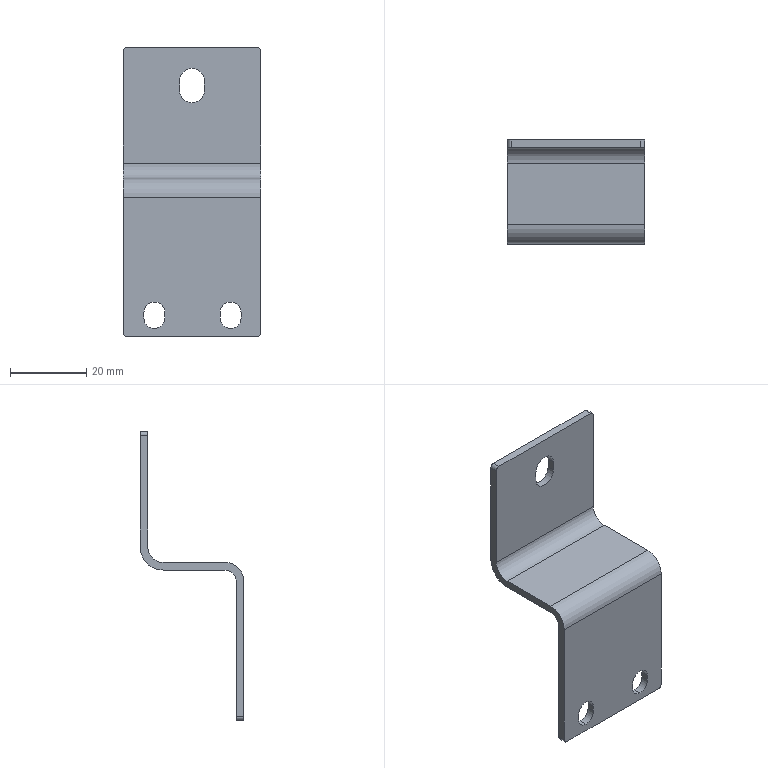Part | NX | features BREP 1 | 1 solid | 33 faces | box 36 x 27.2 x 75.856 mm | volume 6769 mm3 | cylinder 17 | plane 16 | commonest cylinder face diameters 5.5 x6 2 x4 6.5 x3 6 x1 8 x1 10 x1
STEP:
#1=CARTESIAN_POINT('',(427.588,-206.294,1989.75));
#2=VERTEX_POINT('',#1);
#3=CARTESIAN_POINT('',(424.838,-206.294,1987.));
#4=VERTEX_POINT('',#3);
#5=CARTESIAN_POINT('',(424.838,-206.294,1989.75));
#6=DIRECTION('',(0.,1.,0.));
#7=DIRECTION('',(0.,0.,-1.));
#8=AXIS2_PLACEMENT_3D('',#5,#6,#7);
#9=CIRCLE('',#8,2.75);
#10=EDGE_CURVE('',#2,#4,#9,.T.);
#11=ORIENTED_EDGE('',*,*,#10,.T.);
#12=CARTESIAN_POINT('',(424.838,-208.294,1987.));
#13=VERTEX_POINT('',#12);
#14=CARTESIAN_POINT('',(424.838,-206.294,1987.));
#15=DIRECTION('',(0.,-1.,0.));
#16=VECTOR('',#15,1000.);
#17=LINE('',#14,#16);
#18=EDGE_CURVE('',#4,#13,#17,.T.);
#19=ORIENTED_EDGE('',*,*,#18,.T.);
#20=CARTESIAN_POINT('',(427.588,-208.294,1989.75));
#21=VERTEX_POINT('',#20);
#22=CARTESIAN_POINT('',(424.838,-208.294,1989.75));
#23=DIRECTION('',(0.,1.,0.));
#24=DIRECTION('',(0.,0.,-1.));
#25=AXIS2_PLACEMENT_3D('',#22,#23,#24);
#26=CIRCLE('',#25,2.75);
#27=EDGE_CURVE('',#21,#13,#26,.T.);
#28=ORIENTED_EDGE('',*,*,#27,.F.);
#29=CARTESIAN_POINT('',(427.588,-206.294,1989.75));
#30=DIRECTION('',(0.,-1.,0.));
#31=VECTOR('',#30,1000.);
#32=LINE('',#29,#31);
#33=EDGE_CURVE('',#2,#21,#32,.T.);
#34=ORIENTED_EDGE('',*,*,#33,.F.);
#35=EDGE_LOOP('',(#11,#19,#28,#34));
#36=FACE_BOUND('',#35,.T.);
#37=CARTESIAN_POINT('',(424.838,-206.294,1989.75));
#38=DIRECTION('',(0.,-1.,0.));
#39=DIRECTION('',(0.,0.,1.));
#40=AXIS2_PLACEMENT_3D('',#37,#38,#39);
#41=CYLINDRICAL_SURFACE('',#40,2.75);
#42=ADVANCED_FACE('',(#36),#41,.F.);
#43=CARTESIAN_POINT('',(407.588,-206.294,1989.75));
#44=VERTEX_POINT('',#43);
#45=CARTESIAN_POINT('',(404.838,-206.294,1987.));
#46=VERTEX_POINT('',#45);
#47=CARTESIAN_POINT('',(404.838,-206.294,1989.75));
#48=DIRECTION('',(0.,1.,0.));
#49=DIRECTION('',(0.,0.,-1.));
#50=AXIS2_PLACEMENT_3D('',#47,#48,#49);
#51=CIRCLE('',#50,2.75);
#52=EDGE_CURVE('',#44,#46,#51,.T.);
#53=ORIENTED_EDGE('',*,*,#52,.T.);
#54=CARTESIAN_POINT('',(404.838,-208.294,1987.));
#55=VERTEX_POINT('',#54);
#56=CARTESIAN_POINT('',(404.838,-206.294,1987.));
#57=DIRECTION('',(0.,-1.,0.));
#58=VECTOR('',#57,1000.);
#59=LINE('',#56,#58);
#60=EDGE_CURVE('',#46,#55,#59,.T.);
#61=ORIENTED_EDGE('',*,*,#60,.T.);
#62=CARTESIAN_POINT('',(407.588,-208.294,1989.75));
#63=VERTEX_POINT('',#62);
#64=CARTESIAN_POINT('',(404.838,-208.294,1989.75));
#65=DIRECTION('',(0.,1.,0.));
#66=DIRECTION('',(0.,0.,-1.));
#67=AXIS2_PLACEMENT_3D('',#64,#65,#66);
#68=CIRCLE('',#67,2.75);
#69=EDGE_CURVE('',#63,#55,#68,.T.);
#70=ORIENTED_EDGE('',*,*,#69,.F.);
#71=CARTESIAN_POINT('',(407.588,-206.294,1989.75));
#72=DIRECTION('',(0.,-1.,0.));
#73=VECTOR('',#72,1000.);
#74=LINE('',#71,#73);
#75=EDGE_CURVE('',#44,#63,#74,.T.);
#76=ORIENTED_EDGE('',*,*,#75,.F.);
#77=EDGE_LOOP('',(#53,#61,#70,#76));
#78=FACE_BOUND('',#77,.T.);
#79=CARTESIAN_POINT('',(404.838,-206.294,1989.75));
#80=DIRECTION('',(0.,-1.,0.));
#81=DIRECTION('',(0.,0.,1.));
#82=AXIS2_PLACEMENT_3D('',#79,#80,#81);
#83=CYLINDRICAL_SURFACE('',#82,2.75);
#84=ADVANCED_FACE('',(#78),#83,.F.);
#85=CARTESIAN_POINT('',(417.964,-183.094,2052.024));
#86=VERTEX_POINT('',#85);
#87=CARTESIAN_POINT('',(414.714,-183.094,2055.274));
#88=VERTEX_POINT('',#87);
#89=CARTESIAN_POINT('',(414.714,-183.094,2052.024));
#90=DIRECTION('',(0.,-1.,0.));
#91=DIRECTION('',(0.,0.,1.));
#92=AXIS2_PLACEMENT_3D('',#89,#90,#91);
#93=CIRCLE('',#92,3.25);
#94=EDGE_CURVE('',#86,#88,#93,.T.);
#95=ORIENTED_EDGE('',*,*,#94,.T.);
#96=CARTESIAN_POINT('',(414.714,-181.094,2055.274));
#97=VERTEX_POINT('',#96);
#98=CARTESIAN_POINT('',(414.714,-182.594,2055.274));
#99=DIRECTION('',(0.,1.,0.));
#100=VECTOR('',#99,1000.);
#101=LINE('',#98,#100);
#102=EDGE_CURVE('',#88,#97,#101,.T.);
#103=ORIENTED_EDGE('',*,*,#102,.T.);
#104=CARTESIAN_POINT('',(417.964,-181.094,2052.024));
#105=VERTEX_POINT('',#104);
#106=CARTESIAN_POINT('',(414.714,-181.094,2052.024));
#107=DIRECTION('',(0.,-1.,0.));
#108=DIRECTION('',(0.,0.,1.));
#109=AXIS2_PLACEMENT_3D('',#106,#107,#108);
#110=CIRCLE('',#109,3.25);
#111=EDGE_CURVE('',#105,#97,#110,.T.);
#112=ORIENTED_EDGE('',*,*,#111,.F.);
#113=CARTESIAN_POINT('',(417.964,-182.594,2052.024));
#114=DIRECTION('',(0.,1.,0.));
#115=VECTOR('',#114,1000.);
#116=LINE('',#113,#115);
#117=EDGE_CURVE('',#86,#105,#116,.T.);
#118=ORIENTED_EDGE('',*,*,#117,.F.);
#119=EDGE_LOOP('',(#95,#103,#112,#118));
#120=FACE_BOUND('',#119,.T.);
#121=CARTESIAN_POINT('',(414.714,-182.594,2052.024));
#122=DIRECTION('',(0.,1.,0.));
#123=DIRECTION('',(0.,0.,-1.));
#124=AXIS2_PLACEMENT_3D('',#121,#122,#123);
#125=CYLINDRICAL_SURFACE('',#124,3.25);
#126=ADVANCED_FACE('',(#120),#125,.F.);
#127=CARTESIAN_POINT('',(431.713,-206.294,1984.918));
#128=VERTEX_POINT('',#127);
#129=CARTESIAN_POINT('',(432.713,-206.294,1985.918));
#130=VERTEX_POINT('',#129);
#131=CARTESIAN_POINT('',(431.713,-206.294,1985.918));
#132=DIRECTION('',(0.,-1.,0.));
#133=DIRECTION('',(0.,0.,1.));
#134=AXIS2_PLACEMENT_3D('',#131,#132,#133);
#135=CIRCLE('',#134,1.);
#136=EDGE_CURVE('',#128,#130,#135,.T.);
#137=ORIENTED_EDGE('',*,*,#136,.F.);
#138=CARTESIAN_POINT('',(397.713,-206.294,1984.918));
#139=VERTEX_POINT('',#138);
#140=CARTESIAN_POINT('',(1.55,-206.294,1984.918));
#141=DIRECTION('',(1.,0.,0.));
#142=VECTOR('',#141,1000.);
#143=LINE('',#140,#142);
#144=EDGE_CURVE('',#139,#128,#143,.T.);
#145=ORIENTED_EDGE('',*,*,#144,.F.);
#146=CARTESIAN_POINT('',(396.713,-206.294,1985.918));
#147=VERTEX_POINT('',#146);
#148=CARTESIAN_POINT('',(397.713,-206.294,1985.918));
#149=DIRECTION('',(0.,-1.,0.));
#150=DIRECTION('',(0.,0.,1.));
#151=AXIS2_PLACEMENT_3D('',#148,#149,#150);
#152=CIRCLE('',#151,1.);
#153=EDGE_CURVE('',#147,#139,#152,.T.);
#154=ORIENTED_EDGE('',*,*,#153,.F.);
#155=CARTESIAN_POINT('',(396.713,-206.294,2021.418));
#156=VERTEX_POINT('',#155);
#157=CARTESIAN_POINT('',(396.713,-206.294,28.805));
#158=DIRECTION('',(0.,0.,-1.));
#159=VECTOR('',#158,1000.);
#160=LINE('',#157,#159);
#161=EDGE_CURVE('',#156,#147,#160,.T.);
#162=ORIENTED_EDGE('',*,*,#161,.F.);
#163=CARTESIAN_POINT('',(432.713,-206.294,2021.418));
#164=VERTEX_POINT('',#163);
#165=CARTESIAN_POINT('',(1.55,-206.294,2021.418));
#166=DIRECTION('',(-1.,0.,0.));
#167=VECTOR('',#166,1000.);
#168=LINE('',#165,#167);
#169=EDGE_CURVE('',#164,#156,#168,.T.);
#170=ORIENTED_EDGE('',*,*,#169,.F.);
#171=CARTESIAN_POINT('',(432.713,-206.294,28.805));
#172=DIRECTION('',(0.,0.,1.));
#173=VECTOR('',#172,1000.);
#174=LINE('',#171,#173);
#175=EDGE_CURVE('',#130,#164,#174,.T.);
#176=ORIENTED_EDGE('',*,*,#175,.F.);
#177=EDGE_LOOP('',(#137,#145,#154,#162,#170,#176));
#178=FACE_BOUND('',#177,.T.);
#179=CARTESIAN_POINT('',(422.088,-206.294,1991.25));
#180=VERTEX_POINT('',#179);
#181=CARTESIAN_POINT('',(427.588,-206.294,1991.25));
#182=VERTEX_POINT('',#181);
#183=CARTESIAN_POINT('',(424.838,-206.294,1991.25));
#184=DIRECTION('',(0.,1.,0.));
#185=DIRECTION('',(0.,0.,-1.));
#186=AXIS2_PLACEMENT_3D('',#183,#184,#185);
#187=CIRCLE('',#186,2.75);
#188=EDGE_CURVE('',#180,#182,#187,.T.);
#189=ORIENTED_EDGE('',*,*,#188,.F.);
#190=CARTESIAN_POINT('',(422.088,-206.294,1989.75));
#191=VERTEX_POINT('',#190);
#192=CARTESIAN_POINT('',(422.088,-206.294,1991.25));
#193=DIRECTION('',(0.,0.,-1.));
#194=VECTOR('',#193,1000.);
#195=LINE('',#192,#194);
#196=EDGE_CURVE('',#180,#191,#195,.T.);
#197=ORIENTED_EDGE('',*,*,#196,.T.);
#198=CARTESIAN_POINT('',(424.838,-206.294,1989.75));
#199=DIRECTION('',(0.,1.,0.));
#200=DIRECTION('',(0.,0.,-1.));
#201=AXIS2_PLACEMENT_3D('',#198,#199,#200);
#202=CIRCLE('',#201,2.75);
#203=EDGE_CURVE('',#4,#191,#202,.T.);
#204=ORIENTED_EDGE('',*,*,#203,.F.);
#205=ORIENTED_EDGE('',*,*,#10,.F.);
#206=CARTESIAN_POINT('',(427.588,-206.294,1989.75));
#207=DIRECTION('',(0.,0.,1.));
#208=VECTOR('',#207,1000.);
#209=LINE('',#206,#208);
#210=EDGE_CURVE('',#2,#182,#209,.T.);
#211=ORIENTED_EDGE('',*,*,#210,.T.);
#212=EDGE_LOOP('',(#189,#197,#204,#205,#211));
#213=FACE_BOUND('',#212,.T.);
#214=CARTESIAN_POINT('',(402.088,-206.294,1991.25));
#215=VERTEX_POINT('',#214);
#216=CARTESIAN_POINT('',(402.088,-206.294,1989.75));
#217=VERTEX_POINT('',#216);
#218=CARTESIAN_POINT('',(402.088,-206.294,1991.25));
#219=DIRECTION('',(0.,0.,-1.));
#220=VECTOR('',#219,1000.);
#221=LINE('',#218,#220);
#222=EDGE_CURVE('',#215,#217,#221,.T.);
#223=ORIENTED_EDGE('',*,*,#222,.T.);
#224=CARTESIAN_POINT('',(404.838,-206.294,1989.75));
#225=DIRECTION('',(0.,1.,0.));
#226=DIRECTION('',(0.,0.,-1.));
#227=AXIS2_PLACEMENT_3D('',#224,#225,#226);
#228=CIRCLE('',#227,2.75);
#229=EDGE_CURVE('',#46,#217,#228,.T.);
#230=ORIENTED_EDGE('',*,*,#229,.F.);
#231=ORIENTED_EDGE('',*,*,#52,.F.);
#232=CARTESIAN_POINT('',(407.588,-206.294,1991.25));
#233=VERTEX_POINT('',#232);
#234=CARTESIAN_POINT('',(407.588,-206.294,1989.75));
#235=DIRECTION('',(0.,0.,1.));
#236=VECTOR('',#235,1000.);
#237=LINE('',#234,#236);
#238=EDGE_CURVE('',#44,#233,#237,.T.);
#239=ORIENTED_EDGE('',*,*,#238,.T.);
#240=CARTESIAN_POINT('',(404.838,-206.294,1991.25));
#241=DIRECTION('',(0.,1.,0.));
#242=DIRECTION('',(0.,0.,-1.));
#243=AXIS2_PLACEMENT_3D('',#240,#241,#242);
#244=CIRCLE('',#243,2.75);
#245=EDGE_CURVE('',#215,#233,#244,.T.);
#246=ORIENTED_EDGE('',*,*,#245,.F.);
#247=EDGE_LOOP('',(#223,#230,#231,#239,#246));
#248=FACE_BOUND('',#247,.T.);
#249=CARTESIAN_POINT('',(1.55,-206.294,28.805));
#250=DIRECTION('',(0.,-1.,0.));
#251=DIRECTION('',(0.,0.,1.));
#252=AXIS2_PLACEMENT_3D('',#249,#250,#251);
#253=PLANE('',#252);
#254=ADVANCED_FACE('',(#178,#213,#248),#253,.F.);
#255=CARTESIAN_POINT('',(432.713,-203.294,2024.418));
#256=VERTEX_POINT('',#255);
#257=CARTESIAN_POINT('',(432.713,-203.294,2021.418));
#258=DIRECTION('',(1.,0.,0.));
#259=DIRECTION('',(0.,0.,1.));
#260=AXIS2_PLACEMENT_3D('',#257,#258,#259);
#261=CIRCLE('',#260,3.);
#262=EDGE_CURVE('',#256,#164,#261,.T.);
#263=ORIENTED_EDGE('',*,*,#262,.F.);
#264=CARTESIAN_POINT('',(432.713,-187.094,2024.418));
#265=VERTEX_POINT('',#264);
#266=CARTESIAN_POINT('',(432.713,-213.904,2024.418));
#267=DIRECTION('',(0.,-1.,0.));
#268=VECTOR('',#267,1000.);
#269=LINE('',#266,#268);
#270=EDGE_CURVE('',#265,#256,#269,.T.);
#271=ORIENTED_EDGE('',*,*,#270,.F.);
#272=CARTESIAN_POINT('',(432.713,-181.094,2030.418));
#273=VERTEX_POINT('',#272);
#274=CARTESIAN_POINT('',(432.713,-187.094,2030.418));
#275=DIRECTION('',(-1.,0.,0.));
#276=DIRECTION('',(0.,0.,1.));
#277=AXIS2_PLACEMENT_3D('',#274,#275,#276);
#278=CIRCLE('',#277,6.);
#279=EDGE_CURVE('',#273,#265,#278,.T.);
#280=ORIENTED_EDGE('',*,*,#279,.F.);
#281=CARTESIAN_POINT('',(432.713,-181.094,2059.774));
#282=VERTEX_POINT('',#281);
#283=CARTESIAN_POINT('',(432.713,-181.094,1967.823));
#284=DIRECTION('',(0.,0.,-1.));
#285=VECTOR('',#284,1000.);
#286=LINE('',#283,#285);
#287=EDGE_CURVE('',#282,#273,#286,.T.);
#288=ORIENTED_EDGE('',*,*,#287,.F.);
#289=CARTESIAN_POINT('',(432.713,-183.094,2059.774));
#290=VERTEX_POINT('',#289);
#291=CARTESIAN_POINT('',(432.713,-213.904,2059.774));
#292=DIRECTION('',(0.,1.,0.));
#293=VECTOR('',#292,1000.);
#294=LINE('',#291,#293);
#295=EDGE_CURVE('',#290,#282,#294,.T.);
#296=ORIENTED_EDGE('',*,*,#295,.F.);
#297=CARTESIAN_POINT('',(432.713,-183.094,2030.418));
#298=VERTEX_POINT('',#297);
#299=CARTESIAN_POINT('',(432.713,-183.094,1967.823));
#300=DIRECTION('',(0.,0.,1.));
#301=VECTOR('',#300,1000.);
#302=LINE('',#299,#301);
#303=EDGE_CURVE('',#298,#290,#302,.T.);
#304=ORIENTED_EDGE('',*,*,#303,.F.);
#305=CARTESIAN_POINT('',(432.713,-187.094,2026.418));
#306=VERTEX_POINT('',#305);
#307=CARTESIAN_POINT('',(432.713,-187.094,2030.418));
#308=DIRECTION('',(1.,0.,0.));
#309=DIRECTION('',(0.,0.,1.));
#310=AXIS2_PLACEMENT_3D('',#307,#308,#309);
#311=CIRCLE('',#310,4.);
#312=EDGE_CURVE('',#306,#298,#311,.T.);
#313=ORIENTED_EDGE('',*,*,#312,.F.);
#314=CARTESIAN_POINT('',(432.713,-203.294,2026.418));
#315=VERTEX_POINT('',#314);
#316=CARTESIAN_POINT('',(432.713,-213.904,2026.418));
#317=DIRECTION('',(0.,1.,0.));
#318=VECTOR('',#317,1000.);
#319=LINE('',#316,#318);
#320=EDGE_CURVE('',#315,#306,#319,.T.);
#321=ORIENTED_EDGE('',*,*,#320,.F.);
#322=CARTESIAN_POINT('',(432.713,-208.294,2021.418));
#323=VERTEX_POINT('',#322);
#324=CARTESIAN_POINT('',(432.713,-203.294,2021.418));
#325=DIRECTION('',(-1.,0.,0.));
#326=DIRECTION('',(0.,0.,1.));
#327=AXIS2_PLACEMENT_3D('',#324,#325,#326);
#328=CIRCLE('',#327,5.);
#329=EDGE_CURVE('',#323,#315,#328,.T.);
#330=ORIENTED_EDGE('',*,*,#329,.F.);
#331=CARTESIAN_POINT('',(432.713,-208.294,1985.918));
#332=VERTEX_POINT('',#331);
#333=CARTESIAN_POINT('',(432.713,-208.294,1967.823));
#334=DIRECTION('',(0.,0.,1.));
#335=VECTOR('',#334,1000.);
#336=LINE('',#333,#335);
#337=EDGE_CURVE('',#332,#323,#336,.T.);
#338=ORIENTED_EDGE('',*,*,#337,.F.);
#339=CARTESIAN_POINT('',(432.713,-213.904,1985.918));
#340=DIRECTION('',(0.,-1.,0.));
#341=VECTOR('',#340,1000.);
#342=LINE('',#339,#341);
#343=EDGE_CURVE('',#130,#332,#342,.T.);
#344=ORIENTED_EDGE('',*,*,#343,.F.);
#345=ORIENTED_EDGE('',*,*,#175,.T.);
#346=EDGE_LOOP('',(#263,#271,#280,#288,#296,#304,#313,#321,#330,#338,#344,#345));
#347=FACE_BOUND('',#346,.T.);
#348=CARTESIAN_POINT('',(432.713,-213.904,1967.823));
#349=DIRECTION('',(-1.,0.,0.));
#350=DIRECTION('',(0.,0.,-1.));
#351=AXIS2_PLACEMENT_3D('',#348,#349,#350);
#352=PLANE('',#351);
#353=ADVANCED_FACE('',(#347),#352,.F.);
#354=CARTESIAN_POINT('',(397.713,-208.294,1984.918));
#355=VERTEX_POINT('',#354);
#356=CARTESIAN_POINT('',(431.713,-208.294,1984.918));
#357=VERTEX_POINT('',#356);
#358=CARTESIAN_POINT('',(414.713,-208.294,1984.918));
#359=DIRECTION('',(1.,0.,0.));
#360=VECTOR('',#359,1000.);
#361=LINE('',#358,#360);
#362=EDGE_CURVE('',#355,#357,#361,.T.);
#363=ORIENTED_EDGE('',*,*,#362,.F.);
#364=CARTESIAN_POINT('',(397.713,-213.904,1984.918));
#365=DIRECTION('',(0.,-1.,0.));
#366=VECTOR('',#365,1000.);
#367=LINE('',#364,#366);
#368=EDGE_CURVE('',#139,#355,#367,.T.);
#369=ORIENTED_EDGE('',*,*,#368,.F.);
#370=ORIENTED_EDGE('',*,*,#144,.T.);
#371=CARTESIAN_POINT('',(431.713,-213.904,1984.918));
#372=DIRECTION('',(0.,1.,0.));
#373=VECTOR('',#372,1000.);
#374=LINE('',#371,#373);
#375=EDGE_CURVE('',#357,#128,#374,.T.);
#376=ORIENTED_EDGE('',*,*,#375,.F.);
#377=EDGE_LOOP('',(#363,#369,#370,#376));
#378=FACE_BOUND('',#377,.T.);
#379=CARTESIAN_POINT('',(414.713,-213.904,1984.918));
#380=DIRECTION('',(0.,0.,1.));
#381=DIRECTION('',(-1.,0.,0.));
#382=AXIS2_PLACEMENT_3D('',#379,#380,#381);
#383=PLANE('',#382);
#384=ADVANCED_FACE('',(#378),#383,.F.);
#385=CARTESIAN_POINT('',(396.713,-181.094,2059.774));
#386=VERTEX_POINT('',#385);
#387=CARTESIAN_POINT('',(396.713,-181.094,2030.418));
#388=VERTEX_POINT('',#387);
#389=CARTESIAN_POINT('',(396.713,-181.094,1993.823));
#390=DIRECTION('',(0.,0.,-1.));
#391=VECTOR('',#390,1000.);
#392=LINE('',#389,#391);
#393=EDGE_CURVE('',#386,#388,#392,.T.);
#394=ORIENTED_EDGE('',*,*,#393,.T.);
#395=CARTESIAN_POINT('',(396.713,-187.094,2024.418));
#396=VERTEX_POINT('',#395);
#397=CARTESIAN_POINT('',(396.713,-187.094,2030.418));
#398=DIRECTION('',(-1.,0.,0.));
#399=DIRECTION('',(0.,0.,1.));
#400=AXIS2_PLACEMENT_3D('',#397,#398,#399);
#401=CIRCLE('',#400,6.);
#402=EDGE_CURVE('',#388,#396,#401,.T.);
#403=ORIENTED_EDGE('',*,*,#402,.T.);
#404=CARTESIAN_POINT('',(396.713,-203.294,2024.418));
#405=VERTEX_POINT('',#404);
#406=CARTESIAN_POINT('',(396.713,-199.904,2024.418));
#407=DIRECTION('',(0.,-1.,0.));
#408=VECTOR('',#407,1000.);
#409=LINE('',#406,#408);
#410=EDGE_CURVE('',#396,#405,#409,.T.);
#411=ORIENTED_EDGE('',*,*,#410,.T.);
#412=CARTESIAN_POINT('',(396.713,-203.294,2021.418));
#413=DIRECTION('',(1.,0.,0.));
#414=DIRECTION('',(0.,0.,1.));
#415=AXIS2_PLACEMENT_3D('',#412,#413,#414);
#416=CIRCLE('',#415,3.);
#417=EDGE_CURVE('',#405,#156,#416,.T.);
#418=ORIENTED_EDGE('',*,*,#417,.T.);
#419=ORIENTED_EDGE('',*,*,#161,.T.);
#420=CARTESIAN_POINT('',(396.713,-208.294,1985.918));
#421=VERTEX_POINT('',#420);
#422=CARTESIAN_POINT('',(396.713,-199.904,1985.918));
#423=DIRECTION('',(0.,-1.,0.));
#424=VECTOR('',#423,1000.);
#425=LINE('',#422,#424);
#426=EDGE_CURVE('',#147,#421,#425,.T.);
#427=ORIENTED_EDGE('',*,*,#426,.T.);
#428=CARTESIAN_POINT('',(396.713,-208.294,2021.418));
#429=VERTEX_POINT('',#428);
#430=CARTESIAN_POINT('',(396.713,-208.294,1993.823));
#431=DIRECTION('',(0.,0.,1.));
#432=VECTOR('',#431,1000.);
#433=LINE('',#430,#432);
#434=EDGE_CURVE('',#421,#429,#433,.T.);
#435=ORIENTED_EDGE('',*,*,#434,.T.);
#436=CARTESIAN_POINT('',(396.713,-203.294,2026.418));
#437=VERTEX_POINT('',#436);
#438=CARTESIAN_POINT('',(396.713,-203.294,2021.418));
#439=DIRECTION('',(-1.,0.,0.));
#440=DIRECTION('',(0.,0.,1.));
#441=AXIS2_PLACEMENT_3D('',#438,#439,#440);
#442=CIRCLE('',#441,5.);
#443=EDGE_CURVE('',#429,#437,#442,.T.);
#444=ORIENTED_EDGE('',*,*,#443,.T.);
#445=CARTESIAN_POINT('',(396.713,-187.094,2026.418));
#446=VERTEX_POINT('',#445);
#447=CARTESIAN_POINT('',(396.713,-199.904,2026.418));
#448=DIRECTION('',(0.,1.,0.));
#449=VECTOR('',#448,1000.);
#450=LINE('',#447,#449);
#451=EDGE_CURVE('',#437,#446,#450,.T.);
#452=ORIENTED_EDGE('',*,*,#451,.T.);
#453=CARTESIAN_POINT('',(396.713,-183.094,2030.418));
#454=VERTEX_POINT('',#453);
#455=CARTESIAN_POINT('',(396.713,-187.094,2030.418));
#456=DIRECTION('',(1.,0.,0.));
#457=DIRECTION('',(0.,0.,1.));
#458=AXIS2_PLACEMENT_3D('',#455,#456,#457);
#459=CIRCLE('',#458,4.);
#460=EDGE_CURVE('',#446,#454,#459,.T.);
#461=ORIENTED_EDGE('',*,*,#460,.T.);
#462=CARTESIAN_POINT('',(396.713,-183.094,2059.774));
#463=VERTEX_POINT('',#462);
#464=CARTESIAN_POINT('',(396.713,-183.094,1993.823));
#465=DIRECTION('',(0.,0.,1.));
#466=VECTOR('',#465,1000.);
#467=LINE('',#464,#466);
#468=EDGE_CURVE('',#454,#463,#467,.T.);
#469=ORIENTED_EDGE('',*,*,#468,.T.);
#470=CARTESIAN_POINT('',(396.713,-199.904,2059.774));
#471=DIRECTION('',(0.,1.,0.));
#472=VECTOR('',#471,1000.);
#473=LINE('',#470,#472);
#474=EDGE_CURVE('',#463,#386,#473,.T.);
#475=ORIENTED_EDGE('',*,*,#474,.T.);
#476=EDGE_LOOP('',(#394,#403,#411,#418,#419,#427,#435,#444,#452,#461,#469,#475));
#477=FACE_BOUND('',#476,.T.);
#478=CARTESIAN_POINT('',(396.713,-199.904,1993.823));
#479=DIRECTION('',(-1.,0.,0.));
#480=DIRECTION('',(0.,0.,-1.));
#481=AXIS2_PLACEMENT_3D('',#478,#479,#480);
#482=PLANE('',#481);
#483=ADVANCED_FACE('',(#477),#482,.T.);
#484=CARTESIAN_POINT('',(414.727,-203.294,2024.418));
#485=DIRECTION('',(-1.,0.,0.));
#486=VECTOR('',#485,1000.);
#487=LINE('',#484,#486);
#488=EDGE_CURVE('',#256,#405,#487,.T.);
#489=ORIENTED_EDGE('',*,*,#488,.F.);
#490=ORIENTED_EDGE('',*,*,#262,.T.);
#491=ORIENTED_EDGE('',*,*,#169,.T.);
#492=ORIENTED_EDGE('',*,*,#417,.F.);
#493=EDGE_LOOP('',(#489,#490,#491,#492));
#494=FACE_BOUND('',#493,.T.);
#495=CARTESIAN_POINT('',(414.727,-203.294,2021.418));
#496=DIRECTION('',(-1.,0.,0.));
#497=DIRECTION('',(0.,0.,-1.));
#498=AXIS2_PLACEMENT_3D('',#495,#496,#497);
#499=CYLINDRICAL_SURFACE('',#498,3.);
#500=ADVANCED_FACE('',(#494),#499,.F.);
#501=ORIENTED_EDGE('',*,*,#188,.T.);
#502=CARTESIAN_POINT('',(427.588,-208.294,1991.25));
#503=VERTEX_POINT('',#502);
#504=CARTESIAN_POINT('',(427.588,-206.294,1991.25));
#505=DIRECTION('',(0.,1.,0.));
#506=VECTOR('',#505,1000.);
#507=LINE('',#504,#506);
#508=EDGE_CURVE('',#503,#182,#507,.T.);
#509=ORIENTED_EDGE('',*,*,#508,.F.);
#510=CARTESIAN_POINT('',(422.088,-208.294,1991.25));
#511=VERTEX_POINT('',#510);
#512=CARTESIAN_POINT('',(424.838,-208.294,1991.25));
#513=DIRECTION('',(0.,1.,0.));
#514=DIRECTION('',(0.,0.,-1.));
#515=AXIS2_PLACEMENT_3D('',#512,#513,#514);
#516=CIRCLE('',#515,2.75);
#517=EDGE_CURVE('',#511,#503,#516,.T.);
#518=ORIENTED_EDGE('',*,*,#517,.F.);
#519=CARTESIAN_POINT('',(422.088,-206.294,1991.25));
#520=DIRECTION('',(0.,-1.,0.));
#521=VECTOR('',#520,1000.);
#522=LINE('',#519,#521);
#523=EDGE_CURVE('',#180,#511,#522,.T.);
#524=ORIENTED_EDGE('',*,*,#523,.F.);
#525=EDGE_LOOP('',(#501,#509,#518,#524));
#526=FACE_BOUND('',#525,.T.);
#527=CARTESIAN_POINT('',(424.838,-206.294,1991.25));
#528=DIRECTION('',(0.,-1.,0.));
#529=DIRECTION('',(0.,0.,1.));
#530=AXIS2_PLACEMENT_3D('',#527,#528,#529);
#531=CYLINDRICAL_SURFACE('',#530,2.75);
#532=ADVANCED_FACE('',(#526),#531,.F.);
#533=ORIENTED_EDGE('',*,*,#18,.F.);
#534=ORIENTED_EDGE('',*,*,#203,.T.);
#535=CARTESIAN_POINT('',(422.088,-208.294,1989.75));
#536=VERTEX_POINT('',#535);
#537=CARTESIAN_POINT('',(422.088,-206.294,1989.75));
#538=DIRECTION('',(0.,1.,0.));
#539=VECTOR('',#538,1000.);
#540=LINE('',#537,#539);
#541=EDGE_CURVE('',#536,#191,#540,.T.);
#542=ORIENTED_EDGE('',*,*,#541,.F.);
#543=CARTESIAN_POINT('',(424.838,-208.294,1989.75));
#544=DIRECTION('',(0.,1.,0.));
#545=DIRECTION('',(0.,0.,-1.));
#546=AXIS2_PLACEMENT_3D('',#543,#544,#545);
#547=CIRCLE('',#546,2.75);
#548=EDGE_CURVE('',#13,#536,#547,.T.);
#549=ORIENTED_EDGE('',*,*,#548,.F.);
#550=EDGE_LOOP('',(#533,#534,#542,#549));
#551=FACE_BOUND('',#550,.T.);
#552=CARTESIAN_POINT('',(424.838,-206.294,1989.75));
#553=DIRECTION('',(0.,-1.,0.));
#554=DIRECTION('',(0.,0.,1.));
#555=AXIS2_PLACEMENT_3D('',#552,#553,#554);
#556=CYLINDRICAL_SURFACE('',#555,2.75);
#557=ADVANCED_FACE('',(#551),#556,.F.);
#558=ORIENTED_EDGE('',*,*,#245,.T.);
#559=CARTESIAN_POINT('',(407.588,-208.294,1991.25));
#560=VERTEX_POINT('',#559);
#561=CARTESIAN_POINT('',(407.588,-206.294,1991.25));
#562=DIRECTION('',(0.,1.,0.));
#563=VECTOR('',#562,1000.);
#564=LINE('',#561,#563);
#565=EDGE_CURVE('',#560,#233,#564,.T.);
#566=ORIENTED_EDGE('',*,*,#565,.F.);
#567=CARTESIAN_POINT('',(402.088,-208.294,1991.25));
#568=VERTEX_POINT('',#567);
#569=CARTESIAN_POINT('',(404.838,-208.294,1991.25));
#570=DIRECTION('',(0.,1.,0.));
#571=DIRECTION('',(0.,0.,-1.));
#572=AXIS2_PLACEMENT_3D('',#569,#570,#571);
#573=CIRCLE('',#572,2.75);
#574=EDGE_CURVE('',#568,#560,#573,.T.);
#575=ORIENTED_EDGE('',*,*,#574,.F.);
#576=CARTESIAN_POINT('',(402.088,-206.294,1991.25));
#577=DIRECTION('',(0.,-1.,0.));
#578=VECTOR('',#577,1000.);
#579=LINE('',#576,#578);
#580=EDGE_CURVE('',#215,#568,#579,.T.);
#581=ORIENTED_EDGE('',*,*,#580,.F.);
#582=EDGE_LOOP('',(#558,#566,#575,#581));
#583=FACE_BOUND('',#582,.T.);
#584=CARTESIAN_POINT('',(404.838,-206.294,1991.25));
#585=DIRECTION('',(0.,-1.,0.));
#586=DIRECTION('',(0.,0.,1.));
#587=AXIS2_PLACEMENT_3D('',#584,#585,#586);
#588=CYLINDRICAL_SURFACE('',#587,2.75);
#589=ADVANCED_FACE('',(#583),#588,.F.);
#590=ORIENTED_EDGE('',*,*,#60,.F.);
#591=ORIENTED_EDGE('',*,*,#229,.T.);
#592=CARTESIAN_POINT('',(402.088,-208.294,1989.75));
#593=VERTEX_POINT('',#592);
#594=CARTESIAN_POINT('',(402.088,-206.294,1989.75));
#595=DIRECTION('',(0.,1.,0.));
#596=VECTOR('',#595,1000.);
#597=LINE('',#594,#596);
#598=EDGE_CURVE('',#593,#217,#597,.T.);
#599=ORIENTED_EDGE('',*,*,#598,.F.);
#600=CARTESIAN_POINT('',(404.838,-208.294,1989.75));
#601=DIRECTION('',(0.,1.,0.));
#602=DIRECTION('',(0.,0.,-1.));
#603=AXIS2_PLACEMENT_3D('',#600,#601,#602);
#604=CIRCLE('',#603,2.75);
#605=EDGE_CURVE('',#55,#593,#604,.T.);
#606=ORIENTED_EDGE('',*,*,#605,.F.);
#607=EDGE_LOOP('',(#590,#591,#599,#606));
#608=FACE_BOUND('',#607,.T.);
#609=CARTESIAN_POINT('',(404.838,-206.294,1989.75));
#610=DIRECTION('',(0.,-1.,0.));
#611=DIRECTION('',(0.,0.,1.));
#612=AXIS2_PLACEMENT_3D('',#609,#610,#611);
#613=CYLINDRICAL_SURFACE('',#612,2.75);
#614=ADVANCED_FACE('',(#608),#613,.F.);
#615=CARTESIAN_POINT('',(432.713,-187.094,2024.418));
#616=DIRECTION('',(-1.,0.,0.));
#617=VECTOR('',#616,1000.);
#618=LINE('',#615,#617);
#619=EDGE_CURVE('',#265,#396,#618,.T.);
#620=ORIENTED_EDGE('',*,*,#619,.F.);
#621=ORIENTED_EDGE('',*,*,#270,.T.);
#622=ORIENTED_EDGE('',*,*,#488,.T.);
#623=ORIENTED_EDGE('',*,*,#410,.F.);
#624=EDGE_LOOP('',(#620,#621,#622,#623));
#625=FACE_BOUND('',#624,.T.);
#626=CARTESIAN_POINT('',(432.713,-215.404,2024.418));
#627=DIRECTION('',(0.,0.,1.));
#628=DIRECTION('',(-1.,0.,0.));
#629=AXIS2_PLACEMENT_3D('',#626,#627,#628);
#630=PLANE('',#629);
#631=ADVANCED_FACE('',(#625),#630,.F.);
#632=ORIENTED_EDGE('',*,*,#402,.F.);
#633=CARTESIAN_POINT('',(414.713,-181.094,2030.418));
#634=DIRECTION('',(1.,0.,0.));
#635=VECTOR('',#634,1000.);
#636=LINE('',#633,#635);
#637=EDGE_CURVE('',#388,#273,#636,.T.);
#638=ORIENTED_EDGE('',*,*,#637,.T.);
#639=ORIENTED_EDGE('',*,*,#279,.T.);
#640=ORIENTED_EDGE('',*,*,#619,.T.);
#641=EDGE_LOOP('',(#632,#638,#639,#640));
#642=FACE_BOUND('',#641,.T.);
#643=CARTESIAN_POINT('',(414.713,-187.094,2030.418));
#644=DIRECTION('',(-1.,0.,0.));
#645=DIRECTION('',(0.,0.,-1.));
#646=AXIS2_PLACEMENT_3D('',#643,#644,#645);
#647=CYLINDRICAL_SURFACE('',#646,6.);
#648=ADVANCED_FACE('',(#642),#647,.T.);
#649=ORIENTED_EDGE('',*,*,#393,.F.);
#650=CARTESIAN_POINT('',(397.713,-181.094,2060.774));
#651=VERTEX_POINT('',#650);
#652=CARTESIAN_POINT('',(397.713,-181.094,2059.774));
#653=DIRECTION('',(0.,1.,0.));
#654=DIRECTION('',(0.,0.,-1.));
#655=AXIS2_PLACEMENT_3D('',#652,#653,#654);
#656=CIRCLE('',#655,1.);
#657=EDGE_CURVE('',#386,#651,#656,.T.);
#658=ORIENTED_EDGE('',*,*,#657,.T.);
#659=CARTESIAN_POINT('',(431.713,-181.094,2060.774));
#660=VERTEX_POINT('',#659);
#661=CARTESIAN_POINT('',(396.713,-181.094,2060.774));
#662=DIRECTION('',(1.,0.,0.));
#663=VECTOR('',#662,1000.);
#664=LINE('',#661,#663);
#665=EDGE_CURVE('',#651,#660,#664,.T.);
#666=ORIENTED_EDGE('',*,*,#665,.T.);
#667=CARTESIAN_POINT('',(431.713,-181.094,2059.774));
#668=DIRECTION('',(0.,1.,0.));
#669=DIRECTION('',(0.,0.,-1.));
#670=AXIS2_PLACEMENT_3D('',#667,#668,#669);
#671=CIRCLE('',#670,1.);
#672=EDGE_CURVE('',#660,#282,#671,.T.);
#673=ORIENTED_EDGE('',*,*,#672,.T.);
#674=ORIENTED_EDGE('',*,*,#287,.T.);
#675=ORIENTED_EDGE('',*,*,#637,.F.);
#676=EDGE_LOOP('',(#649,#658,#666,#673,#674,#675));
#677=FACE_BOUND('',#676,.T.);
#678=CARTESIAN_POINT('',(411.464,-181.094,2052.024));
#679=VERTEX_POINT('',#678);
#680=CARTESIAN_POINT('',(411.464,-181.094,2049.524));
#681=VERTEX_POINT('',#680);
#682=CARTESIAN_POINT('',(411.464,-181.094,1992.323));
#683=DIRECTION('',(0.,0.,-1.));
#684=VECTOR('',#683,1000.);
#685=LINE('',#682,#684);
#686=EDGE_CURVE('',#679,#681,#685,.T.);
#687=ORIENTED_EDGE('',*,*,#686,.T.);
#688=CARTESIAN_POINT('',(417.964,-181.094,2049.524));
#689=VERTEX_POINT('',#688);
#690=CARTESIAN_POINT('',(414.714,-181.094,2049.524));
#691=DIRECTION('',(0.,-1.,0.));
#692=DIRECTION('',(0.,0.,1.));
#693=AXIS2_PLACEMENT_3D('',#690,#691,#692);
#694=CIRCLE('',#693,3.25);
#695=EDGE_CURVE('',#681,#689,#694,.T.);
#696=ORIENTED_EDGE('',*,*,#695,.T.);
#697=CARTESIAN_POINT('',(417.964,-181.094,1992.323));
#698=DIRECTION('',(0.,0.,1.));
#699=VECTOR('',#698,1000.);
#700=LINE('',#697,#699);
#701=EDGE_CURVE('',#689,#105,#700,.T.);
#702=ORIENTED_EDGE('',*,*,#701,.T.);
#703=ORIENTED_EDGE('',*,*,#111,.T.);
#704=CARTESIAN_POINT('',(414.714,-181.094,2052.024));
#705=DIRECTION('',(0.,-1.,0.));
#706=DIRECTION('',(0.,0.,1.));
#707=AXIS2_PLACEMENT_3D('',#704,#705,#706);
#708=CIRCLE('',#707,3.25);
#709=EDGE_CURVE('',#97,#679,#708,.T.);
#710=ORIENTED_EDGE('',*,*,#709,.T.);
#711=EDGE_LOOP('',(#687,#696,#702,#703,#710));
#712=FACE_BOUND('',#711,.T.);
#713=CARTESIAN_POINT('',(396.713,-181.094,1992.323));
#714=DIRECTION('',(0.,1.,0.));
#715=DIRECTION('',(0.,0.,-1.));
#716=AXIS2_PLACEMENT_3D('',#713,#714,#715);
#717=PLANE('',#716);
#718=ADVANCED_FACE('',(#677,#712),#717,.T.);
#719=CARTESIAN_POINT('',(431.713,-183.094,2060.774));
#720=VERTEX_POINT('',#719);
#721=CARTESIAN_POINT('',(431.713,-195.194,2060.774));
#722=DIRECTION('',(0.,-1.,0.));
#723=VECTOR('',#722,1000.);
#724=LINE('',#721,#723);
#725=EDGE_CURVE('',#660,#720,#724,.T.);
#726=ORIENTED_EDGE('',*,*,#725,.T.);
#727=CARTESIAN_POINT('',(431.713,-183.094,2059.774));
#728=DIRECTION('',(0.,1.,0.));
#729=DIRECTION('',(0.,0.,-1.));
#730=AXIS2_PLACEMENT_3D('',#727,#728,#729);
#731=CIRCLE('',#730,1.);
#732=EDGE_CURVE('',#720,#290,#731,.T.);
#733=ORIENTED_EDGE('',*,*,#732,.T.);
#734=ORIENTED_EDGE('',*,*,#295,.T.);
#735=ORIENTED_EDGE('',*,*,#672,.F.);
#736=EDGE_LOOP('',(#726,#733,#734,#735));
#737=FACE_BOUND('',#736,.T.);
#738=CARTESIAN_POINT('',(431.713,-195.194,2059.774));
#739=DIRECTION('',(0.,-1.,0.));
#740=DIRECTION('',(0.,0.,1.));
#741=AXIS2_PLACEMENT_3D('',#738,#739,#740);
#742=CYLINDRICAL_SURFACE('',#741,1.);
#743=ADVANCED_FACE('',(#737),#742,.T.);
#744=ORIENTED_EDGE('',*,*,#468,.F.);
#745=CARTESIAN_POINT('',(396.713,-183.094,2030.418));
#746=DIRECTION('',(-1.,0.,0.));
#747=VECTOR('',#746,1000.);
#748=LINE('',#745,#747);
#749=EDGE_CURVE('',#298,#454,#748,.T.);
#750=ORIENTED_EDGE('',*,*,#749,.F.);
#751=ORIENTED_EDGE('',*,*,#303,.T.);
#752=ORIENTED_EDGE('',*,*,#732,.F.);
#753=CARTESIAN_POINT('',(397.713,-183.094,2060.774));
#754=VERTEX_POINT('',#753);
#755=CARTESIAN_POINT('',(396.713,-183.094,2060.774));
#756=DIRECTION('',(1.,0.,0.));
#757=VECTOR('',#756,1000.);
#758=LINE('',#755,#757);
#759=EDGE_CURVE('',#754,#720,#758,.T.);
#760=ORIENTED_EDGE('',*,*,#759,.F.);
#761=CARTESIAN_POINT('',(397.713,-183.094,2059.774));
#762=DIRECTION('',(0.,1.,0.));
#763=DIRECTION('',(0.,0.,-1.));
#764=AXIS2_PLACEMENT_3D('',#761,#762,#763);
#765=CIRCLE('',#764,1.);
#766=EDGE_CURVE('',#463,#754,#765,.T.);
#767=ORIENTED_EDGE('',*,*,#766,.F.);
#768=EDGE_LOOP('',(#744,#750,#751,#752,#760,#767));
#769=FACE_BOUND('',#768,.T.);
#770=CARTESIAN_POINT('',(411.464,-183.094,2052.024));
#771=VERTEX_POINT('',#770);
#772=CARTESIAN_POINT('',(411.464,-183.094,2049.524));
#773=VERTEX_POINT('',#772);
#774=CARTESIAN_POINT('',(411.464,-183.094,1992.323));
#775=DIRECTION('',(0.,0.,-1.));
#776=VECTOR('',#775,1000.);
#777=LINE('',#774,#776);
#778=EDGE_CURVE('',#771,#773,#777,.T.);
#779=ORIENTED_EDGE('',*,*,#778,.F.);
#780=CARTESIAN_POINT('',(414.714,-183.094,2052.024));
#781=DIRECTION('',(0.,-1.,0.));
#782=DIRECTION('',(0.,0.,1.));
#783=AXIS2_PLACEMENT_3D('',#780,#781,#782);
#784=CIRCLE('',#783,3.25);
#785=EDGE_CURVE('',#88,#771,#784,.T.);
#786=ORIENTED_EDGE('',*,*,#785,.F.);
#787=ORIENTED_EDGE('',*,*,#94,.F.);
#788=CARTESIAN_POINT('',(417.964,-183.094,2049.524));
#789=VERTEX_POINT('',#788);
#790=CARTESIAN_POINT('',(417.964,-183.094,1992.323));
#791=DIRECTION('',(0.,0.,1.));
#792=VECTOR('',#791,1000.);
#793=LINE('',#790,#792);
#794=EDGE_CURVE('',#789,#86,#793,.T.);
#795=ORIENTED_EDGE('',*,*,#794,.F.);
#796=CARTESIAN_POINT('',(414.714,-183.094,2049.524));
#797=DIRECTION('',(0.,-1.,0.));
#798=DIRECTION('',(0.,0.,1.));
#799=AXIS2_PLACEMENT_3D('',#796,#797,#798);
#800=CIRCLE('',#799,3.25);
#801=EDGE_CURVE('',#773,#789,#800,.T.);
#802=ORIENTED_EDGE('',*,*,#801,.F.);
#803=EDGE_LOOP('',(#779,#786,#787,#795,#802));
#804=FACE_BOUND('',#803,.T.);
#805=CARTESIAN_POINT('',(396.713,-183.094,1992.323));
#806=DIRECTION('',(0.,1.,0.));
#807=DIRECTION('',(0.,0.,-1.));
#808=AXIS2_PLACEMENT_3D('',#805,#806,#807);
#809=PLANE('',#808);
#810=ADVANCED_FACE('',(#769,#804),#809,.F.);
#811=ORIENTED_EDGE('',*,*,#312,.T.);
#812=ORIENTED_EDGE('',*,*,#749,.T.);
#813=ORIENTED_EDGE('',*,*,#460,.F.);
#814=CARTESIAN_POINT('',(414.713,-187.094,2026.418));
#815=DIRECTION('',(-1.,0.,0.));
#816=VECTOR('',#815,1000.);
#817=LINE('',#814,#816);
#818=EDGE_CURVE('',#306,#446,#817,.T.);
#819=ORIENTED_EDGE('',*,*,#818,.F.);
#820=EDGE_LOOP('',(#811,#812,#813,#819));
#821=FACE_BOUND('',#820,.T.);
#822=CARTESIAN_POINT('',(414.713,-187.094,2030.418));
#823=DIRECTION('',(-1.,0.,0.));
#824=DIRECTION('',(0.,0.,-1.));
#825=AXIS2_PLACEMENT_3D('',#822,#823,#824);
#826=CYLINDRICAL_SURFACE('',#825,4.);
#827=ADVANCED_FACE('',(#821),#826,.F.);
#828=CARTESIAN_POINT('',(432.713,-203.294,2026.418));
#829=DIRECTION('',(1.,0.,0.));
#830=VECTOR('',#829,1000.);
#831=LINE('',#828,#830);
#832=EDGE_CURVE('',#437,#315,#831,.T.);
#833=ORIENTED_EDGE('',*,*,#832,.T.);
#834=ORIENTED_EDGE('',*,*,#320,.T.);
#835=ORIENTED_EDGE('',*,*,#818,.T.);
#836=ORIENTED_EDGE('',*,*,#451,.F.);
#837=EDGE_LOOP('',(#833,#834,#835,#836));
#838=FACE_BOUND('',#837,.T.);
#839=CARTESIAN_POINT('',(432.713,-215.404,2026.418));
#840=DIRECTION('',(0.,0.,1.));
#841=DIRECTION('',(-1.,0.,0.));
#842=AXIS2_PLACEMENT_3D('',#839,#840,#841);
#843=PLANE('',#842);
#844=ADVANCED_FACE('',(#838),#843,.T.);
#845=ORIENTED_EDGE('',*,*,#832,.F.);
#846=ORIENTED_EDGE('',*,*,#443,.F.);
#847=CARTESIAN_POINT('',(414.713,-208.294,2021.418));
#848=DIRECTION('',(1.,0.,0.));
#849=VECTOR('',#848,1000.);
#850=LINE('',#847,#849);
#851=EDGE_CURVE('',#429,#323,#850,.T.);
#852=ORIENTED_EDGE('',*,*,#851,.T.);
#853=ORIENTED_EDGE('',*,*,#329,.T.);
#854=EDGE_LOOP('',(#845,#846,#852,#853));
#855=FACE_BOUND('',#854,.T.);
#856=CARTESIAN_POINT('',(414.713,-203.294,2021.418));
#857=DIRECTION('',(-1.,0.,0.));
#858=DIRECTION('',(0.,0.,-1.));
#859=AXIS2_PLACEMENT_3D('',#856,#857,#858);
#860=CYLINDRICAL_SURFACE('',#859,5.);
#861=ADVANCED_FACE('',(#855),#860,.T.);
#862=ORIENTED_EDGE('',*,*,#434,.F.);
#863=CARTESIAN_POINT('',(397.713,-208.294,1985.918));
#864=DIRECTION('',(0.,-1.,0.));
#865=DIRECTION('',(0.,0.,1.));
#866=AXIS2_PLACEMENT_3D('',#863,#864,#865);
#867=CIRCLE('',#866,1.);
#868=EDGE_CURVE('',#421,#355,#867,.T.);
#869=ORIENTED_EDGE('',*,*,#868,.T.);
#870=ORIENTED_EDGE('',*,*,#362,.T.);
#871=CARTESIAN_POINT('',(431.713,-208.294,1985.918));
#872=DIRECTION('',(0.,-1.,0.));
#873=DIRECTION('',(0.,0.,1.));
#874=AXIS2_PLACEMENT_3D('',#871,#872,#873);
#875=CIRCLE('',#874,1.);
#876=EDGE_CURVE('',#357,#332,#875,.T.);
#877=ORIENTED_EDGE('',*,*,#876,.T.);
#878=ORIENTED_EDGE('',*,*,#337,.T.);
#879=ORIENTED_EDGE('',*,*,#851,.F.);
#880=EDGE_LOOP('',(#862,#869,#870,#877,#878,#879));
#881=FACE_BOUND('',#880,.T.);
#882=CARTESIAN_POINT('',(402.088,-208.294,28.805));
#883=DIRECTION('',(0.,0.,1.));
#884=VECTOR('',#883,1000.);
#885=LINE('',#882,#884);
#886=EDGE_CURVE('',#593,#568,#885,.T.);
#887=ORIENTED_EDGE('',*,*,#886,.T.);
#888=ORIENTED_EDGE('',*,*,#574,.T.);
#889=CARTESIAN_POINT('',(407.588,-208.294,28.805));
#890=DIRECTION('',(0.,0.,-1.));
#891=VECTOR('',#890,1000.);
#892=LINE('',#889,#891);
#893=EDGE_CURVE('',#560,#63,#892,.T.);
#894=ORIENTED_EDGE('',*,*,#893,.T.);
#895=ORIENTED_EDGE('',*,*,#69,.T.);
#896=ORIENTED_EDGE('',*,*,#605,.T.);
#897=EDGE_LOOP('',(#887,#888,#894,#895,#896));
#898=FACE_BOUND('',#897,.T.);
#899=ORIENTED_EDGE('',*,*,#517,.T.);
#900=CARTESIAN_POINT('',(427.588,-208.294,28.805));
#901=DIRECTION('',(0.,0.,-1.));
#902=VECTOR('',#901,1000.);
#903=LINE('',#900,#902);
#904=EDGE_CURVE('',#503,#21,#903,.T.);
#905=ORIENTED_EDGE('',*,*,#904,.T.);
#906=ORIENTED_EDGE('',*,*,#27,.T.);
#907=ORIENTED_EDGE('',*,*,#548,.T.);
#908=CARTESIAN_POINT('',(422.088,-208.294,28.805));
#909=DIRECTION('',(0.,0.,1.));
#910=VECTOR('',#909,1000.);
#911=LINE('',#908,#910);
#912=EDGE_CURVE('',#536,#511,#911,.T.);
#913=ORIENTED_EDGE('',*,*,#912,.T.);
#914=EDGE_LOOP('',(#899,#905,#906,#907,#913));
#915=FACE_BOUND('',#914,.T.);
#916=CARTESIAN_POINT('',(1.55,-208.294,28.805));
#917=DIRECTION('',(0.,-1.,0.));
#918=DIRECTION('',(0.,0.,1.));
#919=AXIS2_PLACEMENT_3D('',#916,#917,#918);
#920=PLANE('',#919);
#921=ADVANCED_FACE('',(#881,#898,#915),#920,.T.);
#922=ORIENTED_EDGE('',*,*,#343,.T.);
#923=ORIENTED_EDGE('',*,*,#876,.F.);
#924=ORIENTED_EDGE('',*,*,#375,.T.);
#925=ORIENTED_EDGE('',*,*,#136,.T.);
#926=EDGE_LOOP('',(#922,#923,#924,#925));
#927=FACE_BOUND('',#926,.T.);
#928=CARTESIAN_POINT('',(431.713,-233.919,1985.918));
#929=DIRECTION('',(0.,1.,0.));
#930=DIRECTION('',(0.,0.,-1.));
#931=AXIS2_PLACEMENT_3D('',#928,#929,#930);
#932=CYLINDRICAL_SURFACE('',#931,1.);
#933=ADVANCED_FACE('',(#927),#932,.T.);
#934=ORIENTED_EDGE('',*,*,#426,.F.);
#935=ORIENTED_EDGE('',*,*,#153,.T.);
#936=ORIENTED_EDGE('',*,*,#368,.T.);
#937=ORIENTED_EDGE('',*,*,#868,.F.);
#938=EDGE_LOOP('',(#934,#935,#936,#937));
#939=FACE_BOUND('',#938,.T.);
#940=CARTESIAN_POINT('',(397.713,-233.919,1985.918));
#941=DIRECTION('',(0.,1.,0.));
#942=DIRECTION('',(0.,0.,-1.));
#943=AXIS2_PLACEMENT_3D('',#940,#941,#942);
#944=CYLINDRICAL_SURFACE('',#943,1.);
#945=ADVANCED_FACE('',(#939),#944,.T.);
#946=CARTESIAN_POINT('',(397.713,-195.194,2060.774));
#947=DIRECTION('',(0.,1.,0.));
#948=VECTOR('',#947,1000.);
#949=LINE('',#946,#948);
#950=EDGE_CURVE('',#754,#651,#949,.T.);
#951=ORIENTED_EDGE('',*,*,#950,.T.);
#952=ORIENTED_EDGE('',*,*,#657,.F.);
#953=ORIENTED_EDGE('',*,*,#474,.F.);
#954=ORIENTED_EDGE('',*,*,#766,.T.);
#955=EDGE_LOOP('',(#951,#952,#953,#954));
#956=FACE_BOUND('',#955,.T.);
#957=CARTESIAN_POINT('',(397.713,-195.194,2059.774));
#958=DIRECTION('',(0.,-1.,0.));
#959=DIRECTION('',(0.,0.,1.));
#960=AXIS2_PLACEMENT_3D('',#957,#958,#959);
#961=CYLINDRICAL_SURFACE('',#960,1.);
#962=ADVANCED_FACE('',(#956),#961,.T.);
#963=ORIENTED_EDGE('',*,*,#196,.F.);
#964=ORIENTED_EDGE('',*,*,#523,.T.);
#965=ORIENTED_EDGE('',*,*,#912,.F.);
#966=ORIENTED_EDGE('',*,*,#541,.T.);
#967=EDGE_LOOP('',(#963,#964,#965,#966));
#968=FACE_BOUND('',#967,.T.);
#969=CARTESIAN_POINT('',(422.088,-206.294,1991.25));
#970=DIRECTION('',(-1.,0.,0.));
#971=DIRECTION('',(0.,0.,-1.));
#972=AXIS2_PLACEMENT_3D('',#969,#970,#971);
#973=PLANE('',#972);
#974=ADVANCED_FACE('',(#968),#973,.F.);
#975=ORIENTED_EDGE('',*,*,#904,.F.);
#976=ORIENTED_EDGE('',*,*,#508,.T.);
#977=ORIENTED_EDGE('',*,*,#210,.F.);
#978=ORIENTED_EDGE('',*,*,#33,.T.);
#979=EDGE_LOOP('',(#975,#976,#977,#978));
#980=FACE_BOUND('',#979,.T.);
#981=CARTESIAN_POINT('',(427.588,-206.294,1989.75));
#982=DIRECTION('',(1.,0.,0.));
#983=DIRECTION('',(0.,0.,1.));
#984=AXIS2_PLACEMENT_3D('',#981,#982,#983);
#985=PLANE('',#984);
#986=ADVANCED_FACE('',(#980),#985,.F.);
#987=ORIENTED_EDGE('',*,*,#222,.F.);
#988=ORIENTED_EDGE('',*,*,#580,.T.);
#989=ORIENTED_EDGE('',*,*,#886,.F.);
#990=ORIENTED_EDGE('',*,*,#598,.T.);
#991=EDGE_LOOP('',(#987,#988,#989,#990));
#992=FACE_BOUND('',#991,.T.);
#993=CARTESIAN_POINT('',(402.088,-206.294,1991.25));
#994=DIRECTION('',(-1.,0.,0.));
#995=DIRECTION('',(0.,0.,-1.));
#996=AXIS2_PLACEMENT_3D('',#993,#994,#995);
#997=PLANE('',#996);
#998=ADVANCED_FACE('',(#992),#997,.F.);
#999=ORIENTED_EDGE('',*,*,#238,.F.);
#1000=ORIENTED_EDGE('',*,*,#75,.T.);
#1001=ORIENTED_EDGE('',*,*,#893,.F.);
#1002=ORIENTED_EDGE('',*,*,#565,.T.);
#1003=EDGE_LOOP('',(#999,#1000,#1001,#1002));
#1004=FACE_BOUND('',#1003,.T.);
#1005=CARTESIAN_POINT('',(407.588,-206.294,1989.75));
#1006=DIRECTION('',(1.,0.,0.));
#1007=DIRECTION('',(0.,0.,1.));
#1008=AXIS2_PLACEMENT_3D('',#1005,#1006,#1007);
#1009=PLANE('',#1008);
#1010=ADVANCED_FACE('',(#1004),#1009,.F.);
#1011=ORIENTED_EDGE('',*,*,#725,.F.);
#1012=ORIENTED_EDGE('',*,*,#665,.F.);
#1013=ORIENTED_EDGE('',*,*,#950,.F.);
#1014=ORIENTED_EDGE('',*,*,#759,.T.);
#1015=EDGE_LOOP('',(#1011,#1012,#1013,#1014));
#1016=FACE_BOUND('',#1015,.T.);
#1017=CARTESIAN_POINT('',(414.713,-191.904,2060.774));
#1018=DIRECTION('',(0.,0.,1.));
#1019=DIRECTION('',(-1.,0.,0.));
#1020=AXIS2_PLACEMENT_3D('',#1017,#1018,#1019);
#1021=PLANE('',#1020);
#1022=ADVANCED_FACE('',(#1016),#1021,.T.);
#1023=CARTESIAN_POINT('',(411.464,-182.594,2049.524));
#1024=DIRECTION('',(0.,1.,0.));
#1025=VECTOR('',#1024,1000.);
#1026=LINE('',#1023,#1025);
#1027=EDGE_CURVE('',#773,#681,#1026,.T.);
#1028=ORIENTED_EDGE('',*,*,#1027,.F.);
#1029=ORIENTED_EDGE('',*,*,#801,.T.);
#1030=CARTESIAN_POINT('',(417.964,-182.594,2049.524));
#1031=DIRECTION('',(0.,-1.,0.));
#1032=VECTOR('',#1031,1000.);
#1033=LINE('',#1030,#1032);
#1034=EDGE_CURVE('',#689,#789,#1033,.T.);
#1035=ORIENTED_EDGE('',*,*,#1034,.F.);
#1036=ORIENTED_EDGE('',*,*,#695,.F.);
#1037=EDGE_LOOP('',(#1028,#1029,#1035,#1036));
#1038=FACE_BOUND('',#1037,.T.);
#1039=CARTESIAN_POINT('',(414.714,-182.594,2049.524));
#1040=DIRECTION('',(0.,1.,0.));
#1041=DIRECTION('',(0.,0.,-1.));
#1042=AXIS2_PLACEMENT_3D('',#1039,#1040,#1041);
#1043=CYLINDRICAL_SURFACE('',#1042,3.25);
#1044=ADVANCED_FACE('',(#1038),#1043,.F.);
#1045=ORIENTED_EDGE('',*,*,#686,.F.);
#1046=CARTESIAN_POINT('',(411.464,-184.094,2052.024));
#1047=DIRECTION('',(0.,1.,0.));
#1048=VECTOR('',#1047,1000.);
#1049=LINE('',#1046,#1048);
#1050=EDGE_CURVE('',#771,#679,#1049,.T.);
#1051=ORIENTED_EDGE('',*,*,#1050,.F.);
#1052=ORIENTED_EDGE('',*,*,#778,.T.);
#1053=ORIENTED_EDGE('',*,*,#1027,.T.);
#1054=EDGE_LOOP('',(#1045,#1051,#1052,#1053));
#1055=FACE_BOUND('',#1054,.T.);
#1056=CARTESIAN_POINT('',(411.464,-184.094,2046.274));
#1057=DIRECTION('',(-1.,0.,0.));
#1058=DIRECTION('',(0.,0.,-1.));
#1059=AXIS2_PLACEMENT_3D('',#1056,#1057,#1058);
#1060=PLANE('',#1059);
#1061=ADVANCED_FACE('',(#1055),#1060,.F.);
#1062=ORIENTED_EDGE('',*,*,#102,.F.);
#1063=ORIENTED_EDGE('',*,*,#785,.T.);
#1064=ORIENTED_EDGE('',*,*,#1050,.T.);
#1065=ORIENTED_EDGE('',*,*,#709,.F.);
#1066=EDGE_LOOP('',(#1062,#1063,#1064,#1065));
#1067=FACE_BOUND('',#1066,.T.);
#1068=CARTESIAN_POINT('',(414.714,-182.594,2052.024));
#1069=DIRECTION('',(0.,1.,0.));
#1070=DIRECTION('',(0.,0.,-1.));
#1071=AXIS2_PLACEMENT_3D('',#1068,#1069,#1070);
#1072=CYLINDRICAL_SURFACE('',#1071,3.25);
#1073=ADVANCED_FACE('',(#1067),#1072,.F.);
#1074=ORIENTED_EDGE('',*,*,#794,.T.);
#1075=ORIENTED_EDGE('',*,*,#117,.T.);
#1076=ORIENTED_EDGE('',*,*,#701,.F.);
#1077=ORIENTED_EDGE('',*,*,#1034,.T.);
#1078=EDGE_LOOP('',(#1074,#1075,#1076,#1077));
#1079=FACE_BOUND('',#1078,.T.);
#1080=CARTESIAN_POINT('',(417.964,-184.094,2055.274));
#1081=DIRECTION('',(1.,0.,0.));
#1082=DIRECTION('',(0.,0.,1.));
#1083=AXIS2_PLACEMENT_3D('',#1080,#1081,#1082);
#1084=PLANE('',#1083);
#1085=ADVANCED_FACE('',(#1079),#1084,.F.);
#1086=CLOSED_SHELL('',(#42,#84,#126,#254,#353,#384,#483,#500,#532,#557,#589,#614,#631,#648,#718,#743,#810,#827,#844,#861,#921,#933,#945,#962,#974,#986,#998,#1010,#1022,#1044,#1061,#1073,#1085));
#1087=MANIFOLD_SOLID_BREP('',#1086);
#1088=(LENGTH_UNIT()NAMED_UNIT(*)SI_UNIT(.MILLI.,.METRE.));
#1089=UNCERTAINTY_MEASURE_WITH_UNIT(LENGTH_MEASURE(0.00001),#1088,'','');
#1090=(NAMED_UNIT(*)PLANE_ANGLE_UNIT()SI_UNIT($,.RADIAN.));
#1091=(NAMED_UNIT(*)SI_UNIT($,.STERADIAN.)SOLID_ANGLE_UNIT());
#1092=(GEOMETRIC_REPRESENTATION_CONTEXT(3)GLOBAL_UNCERTAINTY_ASSIGNED_CONTEXT((#1089))GLOBAL_UNIT_ASSIGNED_CONTEXT((#1088,#1090,#1091))REPRESENTATION_CONTEXT('',''));
#1093=ADVANCED_BREP_SHAPE_REPRESENTATION('',(#1087),#1092);